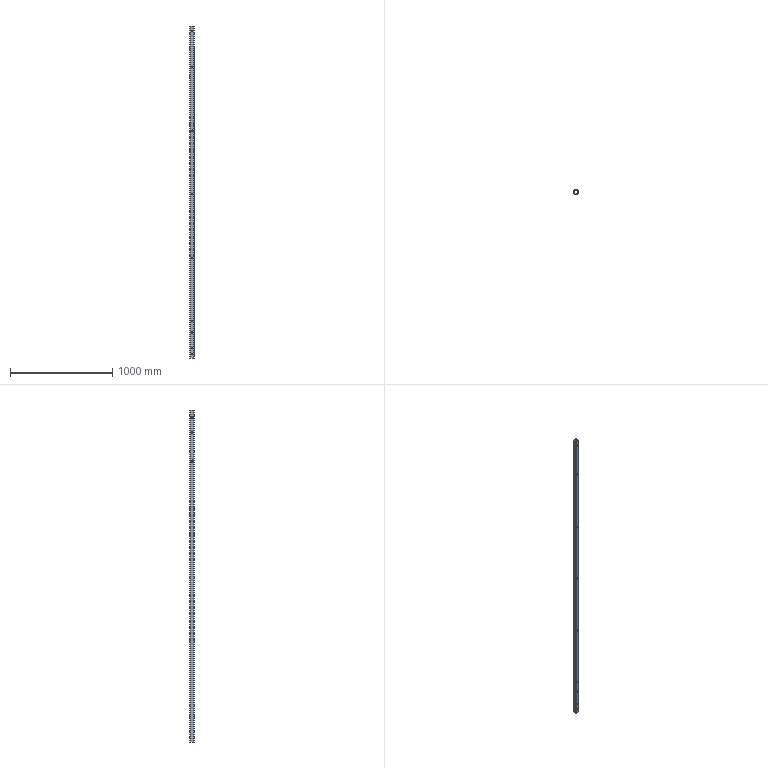Part | STEP file | IN-01-01-04-02 | 1 solid | 78 faces | box 40 x 40 x 3250 mm | volume 1317285 mm3 | cylinder 56 | cone 12 | plane 10 | commonest cylinder face diameters 12.2 x36 17.5 x12 5.8 x4 11.6 x4